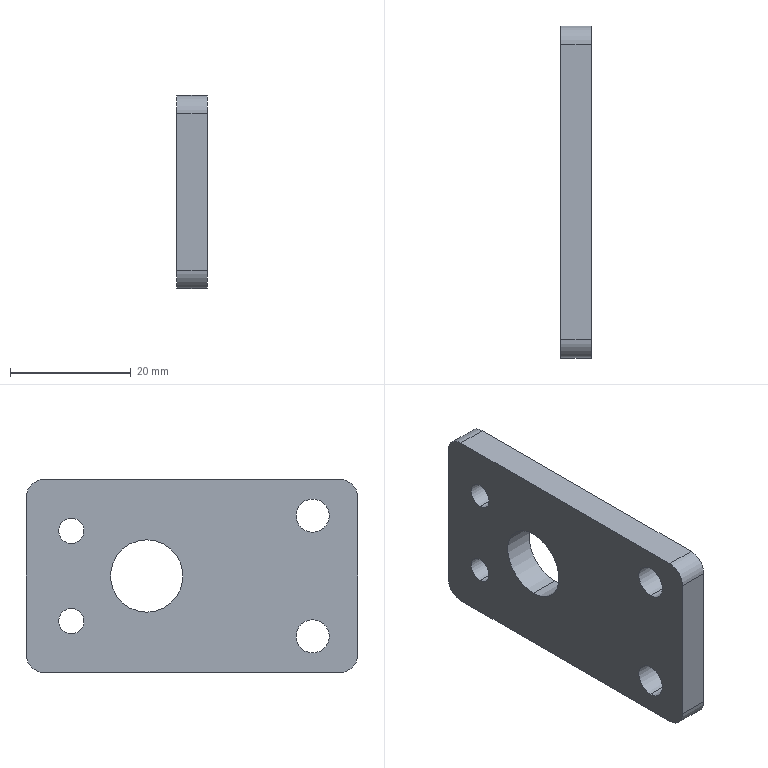Part | SolidWorks | features HoleWzd 2, Cut 1, Fillet 1, FlatPattern 1, SMBaseFlange 1, SheetMetal 1 | 1 solid | 20 faces | box 5 x 55 x 32 mm | volume 7820 mm3 | cylinder 14 | plane 6 | commonest cylinder face diameters 4.2 x4 5.5 x4 6 x4 12 x2
STEP:
#1=CARTESIAN_POINT('',(-5.,7.5,6.));
#2=VERTEX_POINT('',#1);
#3=CARTESIAN_POINT('',(-5.,7.5,-6.));
#4=VERTEX_POINT('',#3);
#5=CARTESIAN_POINT('',(-5.,7.5,0.));
#6=DIRECTION('',(1.,0.,0.));
#7=DIRECTION('',(0.,0.,-1.));
#8=AXIS2_PLACEMENT_3D('',#5,#6,#7);
#9=CIRCLE('',#8,6.);
#10=EDGE_CURVE('',#2,#4,#9,.T.);
#11=ORIENTED_EDGE('',*,*,#10,.F.);
#12=CARTESIAN_POINT('',(0.,7.5,6.));
#13=VERTEX_POINT('',#12);
#14=CARTESIAN_POINT('',(-5.,7.5,6.));
#15=DIRECTION('',(1.,0.,0.));
#16=VECTOR('',#15,1000.);
#17=LINE('',#14,#16);
#18=EDGE_CURVE('',#2,#13,#17,.T.);
#19=ORIENTED_EDGE('',*,*,#18,.T.);
#20=CARTESIAN_POINT('',(0.,7.5,-6.));
#21=VERTEX_POINT('',#20);
#22=CARTESIAN_POINT('',(0.,7.5,0.));
#23=DIRECTION('',(1.,0.,0.));
#24=DIRECTION('',(0.,0.,-1.));
#25=AXIS2_PLACEMENT_3D('',#22,#23,#24);
#26=CIRCLE('',#25,6.);
#27=EDGE_CURVE('',#13,#21,#26,.T.);
#28=ORIENTED_EDGE('',*,*,#27,.T.);
#29=CARTESIAN_POINT('',(-5.,7.5,-6.));
#30=DIRECTION('',(1.,0.,0.));
#31=VECTOR('',#30,1000.);
#32=LINE('',#29,#31);
#33=EDGE_CURVE('',#4,#21,#32,.T.);
#34=ORIENTED_EDGE('',*,*,#33,.F.);
#35=EDGE_LOOP('',(#11,#19,#28,#34));
#36=FACE_OUTER_BOUND('',#35,.T.);
#37=CARTESIAN_POINT('',(-5.,7.5,0.));
#38=DIRECTION('',(1.,0.,0.));
#39=DIRECTION('',(0.,0.,-1.));
#40=AXIS2_PLACEMENT_3D('',#37,#38,#39);
#41=CYLINDRICAL_SURFACE('',#40,6.);
#42=ADVANCED_FACE('',(#36),#41,.F.);
#43=CARTESIAN_POINT('',(0.,20.,-9.6));
#44=VERTEX_POINT('',#43);
#45=CARTESIAN_POINT('',(0.,20.,-5.4));
#46=VERTEX_POINT('',#45);
#47=CARTESIAN_POINT('',(0.,20.,-7.5));
#48=DIRECTION('',(-1.,0.,0.));
#49=DIRECTION('',(0.,0.,1.));
#50=AXIS2_PLACEMENT_3D('',#47,#48,#49);
#51=CIRCLE('',#50,2.1);
#52=EDGE_CURVE('',#44,#46,#51,.T.);
#53=ORIENTED_EDGE('',*,*,#52,.F.);
#54=CARTESIAN_POINT('',(-5.,20.,-9.6));
#55=VERTEX_POINT('',#54);
#56=CARTESIAN_POINT('',(-5.,20.,-9.6));
#57=DIRECTION('',(-1.,0.,0.));
#58=VECTOR('',#57,1000.);
#59=LINE('',#56,#58);
#60=EDGE_CURVE('',#44,#55,#59,.T.);
#61=ORIENTED_EDGE('',*,*,#60,.T.);
#62=CARTESIAN_POINT('',(-5.,20.,-5.4));
#63=VERTEX_POINT('',#62);
#64=CARTESIAN_POINT('',(-5.,20.,-7.5));
#65=DIRECTION('',(-1.,0.,0.));
#66=DIRECTION('',(0.,0.,1.));
#67=AXIS2_PLACEMENT_3D('',#64,#65,#66);
#68=CIRCLE('',#67,2.1);
#69=EDGE_CURVE('',#55,#63,#68,.T.);
#70=ORIENTED_EDGE('',*,*,#69,.T.);
#71=CARTESIAN_POINT('',(-5.,20.,-5.4));
#72=DIRECTION('',(-1.,0.,0.));
#73=VECTOR('',#72,1000.);
#74=LINE('',#71,#73);
#75=EDGE_CURVE('',#46,#63,#74,.T.);
#76=ORIENTED_EDGE('',*,*,#75,.F.);
#77=EDGE_LOOP('',(#53,#61,#70,#76));
#78=FACE_OUTER_BOUND('',#77,.T.);
#79=CARTESIAN_POINT('',(-5.,20.,-7.5));
#80=DIRECTION('',(-1.,0.,0.));
#81=DIRECTION('',(0.,0.,1.));
#82=AXIS2_PLACEMENT_3D('',#79,#80,#81);
#83=CYLINDRICAL_SURFACE('',#82,2.1);
#84=ADVANCED_FACE('',(#78),#83,.F.);
#85=CARTESIAN_POINT('',(0.,20.,5.4));
#86=VERTEX_POINT('',#85);
#87=CARTESIAN_POINT('',(0.,20.,9.6));
#88=VERTEX_POINT('',#87);
#89=CARTESIAN_POINT('',(0.,20.,7.5));
#90=DIRECTION('',(-1.,0.,0.));
#91=DIRECTION('',(0.,0.,1.));
#92=AXIS2_PLACEMENT_3D('',#89,#90,#91);
#93=CIRCLE('',#92,2.1);
#94=EDGE_CURVE('',#86,#88,#93,.T.);
#95=ORIENTED_EDGE('',*,*,#94,.F.);
#96=CARTESIAN_POINT('',(-5.,20.,5.4));
#97=VERTEX_POINT('',#96);
#98=CARTESIAN_POINT('',(-5.,20.,5.4));
#99=DIRECTION('',(-1.,0.,0.));
#100=VECTOR('',#99,1000.);
#101=LINE('',#98,#100);
#102=EDGE_CURVE('',#86,#97,#101,.T.);
#103=ORIENTED_EDGE('',*,*,#102,.T.);
#104=CARTESIAN_POINT('',(-5.,20.,9.6));
#105=VERTEX_POINT('',#104);
#106=CARTESIAN_POINT('',(-5.,20.,7.5));
#107=DIRECTION('',(-1.,0.,0.));
#108=DIRECTION('',(0.,0.,1.));
#109=AXIS2_PLACEMENT_3D('',#106,#107,#108);
#110=CIRCLE('',#109,2.1);
#111=EDGE_CURVE('',#97,#105,#110,.T.);
#112=ORIENTED_EDGE('',*,*,#111,.T.);
#113=CARTESIAN_POINT('',(-5.,20.,9.6));
#114=DIRECTION('',(-1.,0.,0.));
#115=VECTOR('',#114,1000.);
#116=LINE('',#113,#115);
#117=EDGE_CURVE('',#88,#105,#116,.T.);
#118=ORIENTED_EDGE('',*,*,#117,.F.);
#119=EDGE_LOOP('',(#95,#103,#112,#118));
#120=FACE_OUTER_BOUND('',#119,.T.);
#121=CARTESIAN_POINT('',(-5.,20.,7.5));
#122=DIRECTION('',(-1.,0.,0.));
#123=DIRECTION('',(0.,0.,1.));
#124=AXIS2_PLACEMENT_3D('',#121,#122,#123);
#125=CYLINDRICAL_SURFACE('',#124,2.1);
#126=ADVANCED_FACE('',(#120),#125,.F.);
#127=CARTESIAN_POINT('',(-5.,-20.,7.25));
#128=VERTEX_POINT('',#127);
#129=CARTESIAN_POINT('',(-5.,-20.,12.75));
#130=VERTEX_POINT('',#129);
#131=CARTESIAN_POINT('',(-5.,-20.,10.));
#132=DIRECTION('',(-1.,0.,0.));
#133=DIRECTION('',(0.,0.,1.));
#134=AXIS2_PLACEMENT_3D('',#131,#132,#133);
#135=CIRCLE('',#134,2.75);
#136=EDGE_CURVE('',#128,#130,#135,.T.);
#137=ORIENTED_EDGE('',*,*,#136,.T.);
#138=CARTESIAN_POINT('',(0.,-20.,12.75));
#139=VERTEX_POINT('',#138);
#140=CARTESIAN_POINT('',(0.,-20.,12.75));
#141=DIRECTION('',(1.,0.,0.));
#142=VECTOR('',#141,1000.);
#143=LINE('',#140,#142);
#144=EDGE_CURVE('',#130,#139,#143,.T.);
#145=ORIENTED_EDGE('',*,*,#144,.T.);
#146=CARTESIAN_POINT('',(0.,-20.,7.25));
#147=VERTEX_POINT('',#146);
#148=CARTESIAN_POINT('',(0.,-20.,10.));
#149=DIRECTION('',(1.,0.,0.));
#150=DIRECTION('',(0.,0.,-1.));
#151=AXIS2_PLACEMENT_3D('',#148,#149,#150);
#152=CIRCLE('',#151,2.75);
#153=EDGE_CURVE('',#139,#147,#152,.T.);
#154=ORIENTED_EDGE('',*,*,#153,.T.);
#155=CARTESIAN_POINT('',(0.,-20.,7.25));
#156=DIRECTION('',(1.,0.,0.));
#157=VECTOR('',#156,1000.);
#158=LINE('',#155,#157);
#159=EDGE_CURVE('',#128,#147,#158,.T.);
#160=ORIENTED_EDGE('',*,*,#159,.F.);
#161=EDGE_LOOP('',(#137,#145,#154,#160));
#162=FACE_OUTER_BOUND('',#161,.T.);
#163=CARTESIAN_POINT('',(0.,-20.,10.));
#164=DIRECTION('',(1.,0.,0.));
#165=DIRECTION('',(0.,0.,-1.));
#166=AXIS2_PLACEMENT_3D('',#163,#164,#165);
#167=CYLINDRICAL_SURFACE('',#166,2.75);
#168=ADVANCED_FACE('',(#162),#167,.F.);
#169=CARTESIAN_POINT('',(-5.,-20.,-12.75));
#170=VERTEX_POINT('',#169);
#171=CARTESIAN_POINT('',(-5.,-20.,-7.25));
#172=VERTEX_POINT('',#171);
#173=CARTESIAN_POINT('',(-5.,-20.,-10.));
#174=DIRECTION('',(-1.,0.,0.));
#175=DIRECTION('',(0.,0.,1.));
#176=AXIS2_PLACEMENT_3D('',#173,#174,#175);
#177=CIRCLE('',#176,2.75);
#178=EDGE_CURVE('',#170,#172,#177,.T.);
#179=ORIENTED_EDGE('',*,*,#178,.T.);
#180=CARTESIAN_POINT('',(0.,-20.,-7.25));
#181=VERTEX_POINT('',#180);
#182=CARTESIAN_POINT('',(0.,-20.,-7.25));
#183=DIRECTION('',(1.,0.,0.));
#184=VECTOR('',#183,1000.);
#185=LINE('',#182,#184);
#186=EDGE_CURVE('',#172,#181,#185,.T.);
#187=ORIENTED_EDGE('',*,*,#186,.T.);
#188=CARTESIAN_POINT('',(0.,-20.,-12.75));
#189=VERTEX_POINT('',#188);
#190=CARTESIAN_POINT('',(0.,-20.,-10.));
#191=DIRECTION('',(1.,0.,0.));
#192=DIRECTION('',(0.,0.,-1.));
#193=AXIS2_PLACEMENT_3D('',#190,#191,#192);
#194=CIRCLE('',#193,2.75);
#195=EDGE_CURVE('',#181,#189,#194,.T.);
#196=ORIENTED_EDGE('',*,*,#195,.T.);
#197=CARTESIAN_POINT('',(0.,-20.,-12.75));
#198=DIRECTION('',(1.,0.,0.));
#199=VECTOR('',#198,1000.);
#200=LINE('',#197,#199);
#201=EDGE_CURVE('',#170,#189,#200,.T.);
#202=ORIENTED_EDGE('',*,*,#201,.F.);
#203=EDGE_LOOP('',(#179,#187,#196,#202));
#204=FACE_OUTER_BOUND('',#203,.T.);
#205=CARTESIAN_POINT('',(0.,-20.,-10.));
#206=DIRECTION('',(1.,0.,0.));
#207=DIRECTION('',(0.,0.,-1.));
#208=AXIS2_PLACEMENT_3D('',#205,#206,#207);
#209=CYLINDRICAL_SURFACE('',#208,2.75);
#210=ADVANCED_FACE('',(#204),#209,.F.);
#211=CARTESIAN_POINT('',(0.,-24.5,-16.));
#212=VERTEX_POINT('',#211);
#213=CARTESIAN_POINT('',(0.,24.5,-16.));
#214=VERTEX_POINT('',#213);
#215=CARTESIAN_POINT('',(0.,-27.5,-16.));
#216=DIRECTION('',(0.,1.,0.));
#217=VECTOR('',#216,1000.);
#218=LINE('',#215,#217);
#219=EDGE_CURVE('',#212,#214,#218,.T.);
#220=ORIENTED_EDGE('',*,*,#219,.F.);
#221=CARTESIAN_POINT('',(-5.,-24.5,-16.));
#222=VERTEX_POINT('',#221);
#223=CARTESIAN_POINT('',(-5.,-24.5,-16.));
#224=DIRECTION('',(-1.,0.,0.));
#225=VECTOR('',#224,1000.);
#226=LINE('',#223,#225);
#227=EDGE_CURVE('',#212,#222,#226,.T.);
#228=ORIENTED_EDGE('',*,*,#227,.T.);
#229=CARTESIAN_POINT('',(-5.,24.5,-16.));
#230=VERTEX_POINT('',#229);
#231=CARTESIAN_POINT('',(-5.,-27.5,-16.));
#232=DIRECTION('',(0.,1.,0.));
#233=VECTOR('',#232,1000.);
#234=LINE('',#231,#233);
#235=EDGE_CURVE('',#222,#230,#234,.T.);
#236=ORIENTED_EDGE('',*,*,#235,.T.);
#237=CARTESIAN_POINT('',(-5.,24.5,-16.));
#238=DIRECTION('',(1.,0.,0.));
#239=VECTOR('',#238,1000.);
#240=LINE('',#237,#239);
#241=EDGE_CURVE('',#230,#214,#240,.T.);
#242=ORIENTED_EDGE('',*,*,#241,.T.);
#243=EDGE_LOOP('',(#220,#228,#236,#242));
#244=FACE_OUTER_BOUND('',#243,.T.);
#245=CARTESIAN_POINT('',(-5.,-27.5,-16.));
#246=DIRECTION('',(0.,0.,-1.));
#247=DIRECTION('',(-1.,0.,0.));
#248=AXIS2_PLACEMENT_3D('',#245,#246,#247);
#249=PLANE('',#248);
#250=ADVANCED_FACE('',(#244),#249,.T.);
#251=CARTESIAN_POINT('',(-5.,-27.5,13.));
#252=VERTEX_POINT('',#251);
#253=CARTESIAN_POINT('',(-5.,-27.5,-13.));
#254=VERTEX_POINT('',#253);
#255=CARTESIAN_POINT('',(-5.,-27.5,16.));
#256=DIRECTION('',(0.,0.,-1.));
#257=VECTOR('',#256,1000.);
#258=LINE('',#255,#257);
#259=EDGE_CURVE('',#252,#254,#258,.T.);
#260=ORIENTED_EDGE('',*,*,#259,.T.);
#261=CARTESIAN_POINT('',(0.,-27.5,-13.));
#262=VERTEX_POINT('',#261);
#263=CARTESIAN_POINT('',(-5.,-27.5,-13.));
#264=DIRECTION('',(1.,0.,0.));
#265=VECTOR('',#264,1000.);
#266=LINE('',#263,#265);
#267=EDGE_CURVE('',#254,#262,#266,.T.);
#268=ORIENTED_EDGE('',*,*,#267,.T.);
#269=CARTESIAN_POINT('',(0.,-27.5,13.));
#270=VERTEX_POINT('',#269);
#271=CARTESIAN_POINT('',(0.,-27.5,16.));
#272=DIRECTION('',(0.,0.,-1.));
#273=VECTOR('',#272,1000.);
#274=LINE('',#271,#273);
#275=EDGE_CURVE('',#270,#262,#274,.T.);
#276=ORIENTED_EDGE('',*,*,#275,.F.);
#277=CARTESIAN_POINT('',(-5.,-27.5,13.));
#278=DIRECTION('',(-1.,0.,0.));
#279=VECTOR('',#278,1000.);
#280=LINE('',#277,#279);
#281=EDGE_CURVE('',#270,#252,#280,.T.);
#282=ORIENTED_EDGE('',*,*,#281,.T.);
#283=EDGE_LOOP('',(#260,#268,#276,#282));
#284=FACE_OUTER_BOUND('',#283,.T.);
#285=CARTESIAN_POINT('',(-5.,-27.5,16.));
#286=DIRECTION('',(0.,-1.,0.));
#287=DIRECTION('',(0.,0.,-1.));
#288=AXIS2_PLACEMENT_3D('',#285,#286,#287);
#289=PLANE('',#288);
#290=ADVANCED_FACE('',(#284),#289,.T.);
#291=CARTESIAN_POINT('',(-5.,24.5,16.));
#292=VERTEX_POINT('',#291);
#293=CARTESIAN_POINT('',(-5.,-24.5,16.));
#294=VERTEX_POINT('',#293);
#295=CARTESIAN_POINT('',(-5.,-27.5,16.));
#296=DIRECTION('',(0.,-1.,0.));
#297=VECTOR('',#296,1000.);
#298=LINE('',#295,#297);
#299=EDGE_CURVE('',#292,#294,#298,.T.);
#300=ORIENTED_EDGE('',*,*,#299,.T.);
#301=CARTESIAN_POINT('',(0.,-24.5,16.));
#302=VERTEX_POINT('',#301);
#303=CARTESIAN_POINT('',(-5.,-24.5,16.));
#304=DIRECTION('',(1.,0.,0.));
#305=VECTOR('',#304,1000.);
#306=LINE('',#303,#305);
#307=EDGE_CURVE('',#294,#302,#306,.T.);
#308=ORIENTED_EDGE('',*,*,#307,.T.);
#309=CARTESIAN_POINT('',(0.,24.5,16.));
#310=VERTEX_POINT('',#309);
#311=CARTESIAN_POINT('',(0.,-27.5,16.));
#312=DIRECTION('',(0.,-1.,0.));
#313=VECTOR('',#312,1000.);
#314=LINE('',#311,#313);
#315=EDGE_CURVE('',#310,#302,#314,.T.);
#316=ORIENTED_EDGE('',*,*,#315,.F.);
#317=CARTESIAN_POINT('',(-5.,24.5,16.));
#318=DIRECTION('',(-1.,0.,0.));
#319=VECTOR('',#318,1000.);
#320=LINE('',#317,#319);
#321=EDGE_CURVE('',#310,#292,#320,.T.);
#322=ORIENTED_EDGE('',*,*,#321,.T.);
#323=EDGE_LOOP('',(#300,#308,#316,#322));
#324=FACE_OUTER_BOUND('',#323,.T.);
#325=CARTESIAN_POINT('',(-5.,-27.5,16.));
#326=DIRECTION('',(0.,0.,1.));
#327=DIRECTION('',(1.,0.,0.));
#328=AXIS2_PLACEMENT_3D('',#325,#326,#327);
#329=PLANE('',#328);
#330=ADVANCED_FACE('',(#324),#329,.T.);
#331=CARTESIAN_POINT('',(0.,27.5,-13.));
#332=VERTEX_POINT('',#331);
#333=CARTESIAN_POINT('',(0.,27.5,13.));
#334=VERTEX_POINT('',#333);
#335=CARTESIAN_POINT('',(0.,27.5,16.));
#336=DIRECTION('',(0.,0.,1.));
#337=VECTOR('',#336,1000.);
#338=LINE('',#335,#337);
#339=EDGE_CURVE('',#332,#334,#338,.T.);
#340=ORIENTED_EDGE('',*,*,#339,.F.);
#341=CARTESIAN_POINT('',(-5.,27.5,-13.));
#342=VERTEX_POINT('',#341);
#343=CARTESIAN_POINT('',(-5.,27.5,-13.));
#344=DIRECTION('',(-1.,0.,0.));
#345=VECTOR('',#344,1000.);
#346=LINE('',#343,#345);
#347=EDGE_CURVE('',#332,#342,#346,.T.);
#348=ORIENTED_EDGE('',*,*,#347,.T.);
#349=CARTESIAN_POINT('',(-5.,27.5,13.));
#350=VERTEX_POINT('',#349);
#351=CARTESIAN_POINT('',(-5.,27.5,16.));
#352=DIRECTION('',(0.,0.,1.));
#353=VECTOR('',#352,1000.);
#354=LINE('',#351,#353);
#355=EDGE_CURVE('',#342,#350,#354,.T.);
#356=ORIENTED_EDGE('',*,*,#355,.T.);
#357=CARTESIAN_POINT('',(-5.,27.5,13.));
#358=DIRECTION('',(1.,0.,0.));
#359=VECTOR('',#358,1000.);
#360=LINE('',#357,#359);
#361=EDGE_CURVE('',#350,#334,#360,.T.);
#362=ORIENTED_EDGE('',*,*,#361,.T.);
#363=EDGE_LOOP('',(#340,#348,#356,#362));
#364=FACE_OUTER_BOUND('',#363,.T.);
#365=CARTESIAN_POINT('',(-5.,27.5,16.));
#366=DIRECTION('',(0.,1.,0.));
#367=DIRECTION('',(0.,0.,1.));
#368=AXIS2_PLACEMENT_3D('',#365,#366,#367);
#369=PLANE('',#368);
#370=ADVANCED_FACE('',(#364),#369,.T.);
#371=CARTESIAN_POINT('',(-5.,7.5,0.));
#372=DIRECTION('',(1.,0.,0.));
#373=DIRECTION('',(0.,0.,-1.));
#374=AXIS2_PLACEMENT_3D('',#371,#372,#373);
#375=CIRCLE('',#374,6.);
#376=EDGE_CURVE('',#4,#2,#375,.T.);
#377=ORIENTED_EDGE('',*,*,#376,.T.);
#378=ORIENTED_EDGE('',*,*,#10,.T.);
#379=EDGE_LOOP('',(#377,#378));
#380=FACE_BOUND('',#379,.T.);
#381=CARTESIAN_POINT('',(-5.,20.,-7.5));
#382=DIRECTION('',(-1.,0.,0.));
#383=DIRECTION('',(0.,0.,1.));
#384=AXIS2_PLACEMENT_3D('',#381,#382,#383);
#385=CIRCLE('',#384,2.1);
#386=EDGE_CURVE('',#63,#55,#385,.T.);
#387=ORIENTED_EDGE('',*,*,#386,.F.);
#388=ORIENTED_EDGE('',*,*,#69,.F.);
#389=EDGE_LOOP('',(#387,#388));
#390=FACE_BOUND('',#389,.T.);
#391=CARTESIAN_POINT('',(-5.,20.,7.5));
#392=DIRECTION('',(-1.,0.,0.));
#393=DIRECTION('',(0.,0.,1.));
#394=AXIS2_PLACEMENT_3D('',#391,#392,#393);
#395=CIRCLE('',#394,2.1);
#396=EDGE_CURVE('',#105,#97,#395,.T.);
#397=ORIENTED_EDGE('',*,*,#396,.F.);
#398=ORIENTED_EDGE('',*,*,#111,.F.);
#399=EDGE_LOOP('',(#397,#398));
#400=FACE_BOUND('',#399,.T.);
#401=ORIENTED_EDGE('',*,*,#136,.F.);
#402=CARTESIAN_POINT('',(-5.,-20.,10.));
#403=DIRECTION('',(-1.,0.,0.));
#404=DIRECTION('',(0.,0.,1.));
#405=AXIS2_PLACEMENT_3D('',#402,#403,#404);
#406=CIRCLE('',#405,2.75);
#407=EDGE_CURVE('',#130,#128,#406,.T.);
#408=ORIENTED_EDGE('',*,*,#407,.F.);
#409=EDGE_LOOP('',(#401,#408));
#410=FACE_BOUND('',#409,.T.);
#411=ORIENTED_EDGE('',*,*,#178,.F.);
#412=CARTESIAN_POINT('',(-5.,-20.,-10.));
#413=DIRECTION('',(-1.,0.,0.));
#414=DIRECTION('',(0.,0.,1.));
#415=AXIS2_PLACEMENT_3D('',#412,#413,#414);
#416=CIRCLE('',#415,2.75);
#417=EDGE_CURVE('',#172,#170,#416,.T.);
#418=ORIENTED_EDGE('',*,*,#417,.F.);
#419=EDGE_LOOP('',(#411,#418));
#420=FACE_BOUND('',#419,.T.);
#421=ORIENTED_EDGE('',*,*,#235,.F.);
#422=CARTESIAN_POINT('',(-5.,-24.5,-13.));
#423=DIRECTION('',(-1.,0.,0.));
#424=DIRECTION('',(0.,0.,1.));
#425=AXIS2_PLACEMENT_3D('',#422,#423,#424);
#426=CIRCLE('',#425,3.);
#427=EDGE_CURVE('',#222,#254,#426,.T.);
#428=ORIENTED_EDGE('',*,*,#427,.T.);
#429=ORIENTED_EDGE('',*,*,#259,.F.);
#430=CARTESIAN_POINT('',(-5.,-24.5,13.));
#431=DIRECTION('',(-1.,0.,0.));
#432=DIRECTION('',(0.,0.,1.));
#433=AXIS2_PLACEMENT_3D('',#430,#431,#432);
#434=CIRCLE('',#433,3.);
#435=EDGE_CURVE('',#252,#294,#434,.T.);
#436=ORIENTED_EDGE('',*,*,#435,.T.);
#437=ORIENTED_EDGE('',*,*,#299,.F.);
#438=CARTESIAN_POINT('',(-5.,24.5,13.));
#439=DIRECTION('',(-1.,0.,0.));
#440=DIRECTION('',(0.,0.,1.));
#441=AXIS2_PLACEMENT_3D('',#438,#439,#440);
#442=CIRCLE('',#441,3.);
#443=EDGE_CURVE('',#292,#350,#442,.T.);
#444=ORIENTED_EDGE('',*,*,#443,.T.);
#445=ORIENTED_EDGE('',*,*,#355,.F.);
#446=CARTESIAN_POINT('',(-5.,24.5,-13.));
#447=DIRECTION('',(-1.,0.,0.));
#448=DIRECTION('',(0.,0.,1.));
#449=AXIS2_PLACEMENT_3D('',#446,#447,#448);
#450=CIRCLE('',#449,3.);
#451=EDGE_CURVE('',#342,#230,#450,.T.);
#452=ORIENTED_EDGE('',*,*,#451,.T.);
#453=EDGE_LOOP('',(#421,#428,#429,#436,#437,#444,#445,#452));
#454=FACE_OUTER_BOUND('',#453,.T.);
#455=CARTESIAN_POINT('',(-5.,0.,0.));
#456=DIRECTION('',(-1.,0.,0.));
#457=DIRECTION('',(0.,0.,1.));
#458=AXIS2_PLACEMENT_3D('',#455,#456,#457);
#459=PLANE('',#458);
#460=ADVANCED_FACE('',(#380,#390,#400,#410,#420,#454),#459,.T.);
#461=CARTESIAN_POINT('',(0.,7.5,0.));
#462=DIRECTION('',(1.,0.,0.));
#463=DIRECTION('',(0.,0.,-1.));
#464=AXIS2_PLACEMENT_3D('',#461,#462,#463);
#465=CIRCLE('',#464,6.);
#466=EDGE_CURVE('',#21,#13,#465,.T.);
#467=ORIENTED_EDGE('',*,*,#466,.F.);
#468=ORIENTED_EDGE('',*,*,#27,.F.);
#469=EDGE_LOOP('',(#467,#468));
#470=FACE_BOUND('',#469,.T.);
#471=CARTESIAN_POINT('',(0.,20.,-7.5));
#472=DIRECTION('',(-1.,0.,0.));
#473=DIRECTION('',(0.,0.,1.));
#474=AXIS2_PLACEMENT_3D('',#471,#472,#473);
#475=CIRCLE('',#474,2.1);
#476=EDGE_CURVE('',#46,#44,#475,.T.);
#477=ORIENTED_EDGE('',*,*,#476,.T.);
#478=ORIENTED_EDGE('',*,*,#52,.T.);
#479=EDGE_LOOP('',(#477,#478));
#480=FACE_BOUND('',#479,.T.);
#481=CARTESIAN_POINT('',(0.,20.,7.5));
#482=DIRECTION('',(-1.,0.,0.));
#483=DIRECTION('',(0.,0.,1.));
#484=AXIS2_PLACEMENT_3D('',#481,#482,#483);
#485=CIRCLE('',#484,2.1);
#486=EDGE_CURVE('',#88,#86,#485,.T.);
#487=ORIENTED_EDGE('',*,*,#486,.T.);
#488=ORIENTED_EDGE('',*,*,#94,.T.);
#489=EDGE_LOOP('',(#487,#488));
#490=FACE_BOUND('',#489,.T.);
#491=CARTESIAN_POINT('',(0.,-20.,10.));
#492=DIRECTION('',(1.,0.,0.));
#493=DIRECTION('',(0.,0.,-1.));
#494=AXIS2_PLACEMENT_3D('',#491,#492,#493);
#495=CIRCLE('',#494,2.75);
#496=EDGE_CURVE('',#147,#139,#495,.T.);
#497=ORIENTED_EDGE('',*,*,#496,.F.);
#498=ORIENTED_EDGE('',*,*,#153,.F.);
#499=EDGE_LOOP('',(#497,#498));
#500=FACE_BOUND('',#499,.T.);
#501=CARTESIAN_POINT('',(0.,-20.,-10.));
#502=DIRECTION('',(1.,0.,0.));
#503=DIRECTION('',(0.,0.,-1.));
#504=AXIS2_PLACEMENT_3D('',#501,#502,#503);
#505=CIRCLE('',#504,2.75);
#506=EDGE_CURVE('',#189,#181,#505,.T.);
#507=ORIENTED_EDGE('',*,*,#506,.F.);
#508=ORIENTED_EDGE('',*,*,#195,.F.);
#509=EDGE_LOOP('',(#507,#508));
#510=FACE_BOUND('',#509,.T.);
#511=ORIENTED_EDGE('',*,*,#275,.T.);
#512=CARTESIAN_POINT('',(0.,-24.5,-13.));
#513=DIRECTION('',(1.,0.,0.));
#514=DIRECTION('',(0.,0.,1.));
#515=AXIS2_PLACEMENT_3D('',#512,#513,#514);
#516=CIRCLE('',#515,3.);
#517=EDGE_CURVE('',#262,#212,#516,.T.);
#518=ORIENTED_EDGE('',*,*,#517,.T.);
#519=ORIENTED_EDGE('',*,*,#219,.T.);
#520=CARTESIAN_POINT('',(0.,24.5,-13.));
#521=DIRECTION('',(1.,0.,0.));
#522=DIRECTION('',(0.,0.,1.));
#523=AXIS2_PLACEMENT_3D('',#520,#521,#522);
#524=CIRCLE('',#523,3.);
#525=EDGE_CURVE('',#214,#332,#524,.T.);
#526=ORIENTED_EDGE('',*,*,#525,.T.);
#527=ORIENTED_EDGE('',*,*,#339,.T.);
#528=CARTESIAN_POINT('',(0.,24.5,13.));
#529=DIRECTION('',(1.,0.,0.));
#530=DIRECTION('',(0.,0.,1.));
#531=AXIS2_PLACEMENT_3D('',#528,#529,#530);
#532=CIRCLE('',#531,3.);
#533=EDGE_CURVE('',#334,#310,#532,.T.);
#534=ORIENTED_EDGE('',*,*,#533,.T.);
#535=ORIENTED_EDGE('',*,*,#315,.T.);
#536=CARTESIAN_POINT('',(0.,-24.5,13.));
#537=DIRECTION('',(1.,0.,0.));
#538=DIRECTION('',(0.,0.,1.));
#539=AXIS2_PLACEMENT_3D('',#536,#537,#538);
#540=CIRCLE('',#539,3.);
#541=EDGE_CURVE('',#302,#270,#540,.T.);
#542=ORIENTED_EDGE('',*,*,#541,.T.);
#543=EDGE_LOOP('',(#511,#518,#519,#526,#527,#534,#535,#542));
#544=FACE_OUTER_BOUND('',#543,.T.);
#545=CARTESIAN_POINT('',(0.,0.,0.));
#546=DIRECTION('',(-1.,0.,0.));
#547=DIRECTION('',(0.,0.,1.));
#548=AXIS2_PLACEMENT_3D('',#545,#546,#547);
#549=PLANE('',#548);
#550=ADVANCED_FACE('',(#470,#480,#490,#500,#510,#544),#549,.F.);
#551=ORIENTED_EDGE('',*,*,#186,.F.);
#552=ORIENTED_EDGE('',*,*,#417,.T.);
#553=ORIENTED_EDGE('',*,*,#201,.T.);
#554=ORIENTED_EDGE('',*,*,#506,.T.);
#555=EDGE_LOOP('',(#551,#552,#553,#554));
#556=FACE_OUTER_BOUND('',#555,.T.);
#557=CARTESIAN_POINT('',(0.,-20.,-10.));
#558=DIRECTION('',(1.,0.,0.));
#559=DIRECTION('',(0.,0.,-1.));
#560=AXIS2_PLACEMENT_3D('',#557,#558,#559);
#561=CYLINDRICAL_SURFACE('',#560,2.75);
#562=ADVANCED_FACE('',(#556),#561,.F.);
#563=ORIENTED_EDGE('',*,*,#144,.F.);
#564=ORIENTED_EDGE('',*,*,#407,.T.);
#565=ORIENTED_EDGE('',*,*,#159,.T.);
#566=ORIENTED_EDGE('',*,*,#496,.T.);
#567=EDGE_LOOP('',(#563,#564,#565,#566));
#568=FACE_OUTER_BOUND('',#567,.T.);
#569=CARTESIAN_POINT('',(0.,-20.,10.));
#570=DIRECTION('',(1.,0.,0.));
#571=DIRECTION('',(0.,0.,-1.));
#572=AXIS2_PLACEMENT_3D('',#569,#570,#571);
#573=CYLINDRICAL_SURFACE('',#572,2.75);
#574=ADVANCED_FACE('',(#568),#573,.F.);
#575=ORIENTED_EDGE('',*,*,#102,.F.);
#576=ORIENTED_EDGE('',*,*,#486,.F.);
#577=ORIENTED_EDGE('',*,*,#117,.T.);
#578=ORIENTED_EDGE('',*,*,#396,.T.);
#579=EDGE_LOOP('',(#575,#576,#577,#578));
#580=FACE_OUTER_BOUND('',#579,.T.);
#581=CARTESIAN_POINT('',(-5.,20.,7.5));
#582=DIRECTION('',(-1.,0.,0.));
#583=DIRECTION('',(0.,0.,1.));
#584=AXIS2_PLACEMENT_3D('',#581,#582,#583);
#585=CYLINDRICAL_SURFACE('',#584,2.1);
#586=ADVANCED_FACE('',(#580),#585,.F.);
#587=ORIENTED_EDGE('',*,*,#60,.F.);
#588=ORIENTED_EDGE('',*,*,#476,.F.);
#589=ORIENTED_EDGE('',*,*,#75,.T.);
#590=ORIENTED_EDGE('',*,*,#386,.T.);
#591=EDGE_LOOP('',(#587,#588,#589,#590));
#592=FACE_OUTER_BOUND('',#591,.T.);
#593=CARTESIAN_POINT('',(-5.,20.,-7.5));
#594=DIRECTION('',(-1.,0.,0.));
#595=DIRECTION('',(0.,0.,1.));
#596=AXIS2_PLACEMENT_3D('',#593,#594,#595);
#597=CYLINDRICAL_SURFACE('',#596,2.1);
#598=ADVANCED_FACE('',(#592),#597,.F.);
#599=ORIENTED_EDGE('',*,*,#427,.F.);
#600=ORIENTED_EDGE('',*,*,#227,.F.);
#601=ORIENTED_EDGE('',*,*,#517,.F.);
#602=ORIENTED_EDGE('',*,*,#267,.F.);
#603=EDGE_LOOP('',(#599,#600,#601,#602));
#604=FACE_OUTER_BOUND('',#603,.T.);
#605=CARTESIAN_POINT('',(-5.,-24.5,-13.));
#606=DIRECTION('',(1.,0.,0.));
#607=DIRECTION('',(0.,0.,-1.));
#608=AXIS2_PLACEMENT_3D('',#605,#606,#607);
#609=CYLINDRICAL_SURFACE('',#608,3.);
#610=ADVANCED_FACE('',(#604),#609,.T.);
#611=ORIENTED_EDGE('',*,*,#435,.F.);
#612=ORIENTED_EDGE('',*,*,#281,.F.);
#613=ORIENTED_EDGE('',*,*,#541,.F.);
#614=ORIENTED_EDGE('',*,*,#307,.F.);
#615=EDGE_LOOP('',(#611,#612,#613,#614));
#616=FACE_OUTER_BOUND('',#615,.T.);
#617=CARTESIAN_POINT('',(-5.,-24.5,13.));
#618=DIRECTION('',(1.,0.,0.));
#619=DIRECTION('',(0.,0.,-1.));
#620=AXIS2_PLACEMENT_3D('',#617,#618,#619);
#621=CYLINDRICAL_SURFACE('',#620,3.);
#622=ADVANCED_FACE('',(#616),#621,.T.);
#623=ORIENTED_EDGE('',*,*,#451,.F.);
#624=ORIENTED_EDGE('',*,*,#347,.F.);
#625=ORIENTED_EDGE('',*,*,#525,.F.);
#626=ORIENTED_EDGE('',*,*,#241,.F.);
#627=EDGE_LOOP('',(#623,#624,#625,#626));
#628=FACE_OUTER_BOUND('',#627,.T.);
#629=CARTESIAN_POINT('',(-5.,24.5,-13.));
#630=DIRECTION('',(1.,0.,0.));
#631=DIRECTION('',(0.,0.,-1.));
#632=AXIS2_PLACEMENT_3D('',#629,#630,#631);
#633=CYLINDRICAL_SURFACE('',#632,3.);
#634=ADVANCED_FACE('',(#628),#633,.T.);
#635=ORIENTED_EDGE('',*,*,#443,.F.);
#636=ORIENTED_EDGE('',*,*,#321,.F.);
#637=ORIENTED_EDGE('',*,*,#533,.F.);
#638=ORIENTED_EDGE('',*,*,#361,.F.);
#639=EDGE_LOOP('',(#635,#636,#637,#638));
#640=FACE_OUTER_BOUND('',#639,.T.);
#641=CARTESIAN_POINT('',(-5.,24.5,13.));
#642=DIRECTION('',(1.,0.,0.));
#643=DIRECTION('',(0.,0.,-1.));
#644=AXIS2_PLACEMENT_3D('',#641,#642,#643);
#645=CYLINDRICAL_SURFACE('',#644,3.);
#646=ADVANCED_FACE('',(#640),#645,.T.);
#647=ORIENTED_EDGE('',*,*,#18,.F.);
#648=ORIENTED_EDGE('',*,*,#376,.F.);
#649=ORIENTED_EDGE('',*,*,#33,.T.);
#650=ORIENTED_EDGE('',*,*,#466,.T.);
#651=EDGE_LOOP('',(#647,#648,#649,#650));
#652=FACE_OUTER_BOUND('',#651,.T.);
#653=CARTESIAN_POINT('',(-5.,7.5,0.));
#654=DIRECTION('',(1.,0.,0.));
#655=DIRECTION('',(0.,0.,-1.));
#656=AXIS2_PLACEMENT_3D('',#653,#654,#655);
#657=CYLINDRICAL_SURFACE('',#656,6.);
#658=ADVANCED_FACE('',(#652),#657,.F.);
#659=CLOSED_SHELL('',(#42,#84,#126,#168,#210,#250,#290,#330,#370,#460,#550,#562,#574,#586,#598,#610,#622,#634,#646,#658));
#660=MANIFOLD_SOLID_BREP('',#659);
#661=CARTESIAN_POINT('',(0.,0.,0.));
#662=DIRECTION('',(0.,0.,1.));
#663=DIRECTION('',(1.,0.,0.));
#664=AXIS2_PLACEMENT_3D('',#661,#662,#663);
#665=(LENGTH_UNIT()NAMED_UNIT(*)SI_UNIT(.MILLI.,.METRE.));
#666=UNCERTAINTY_MEASURE_WITH_UNIT(LENGTH_MEASURE(0.00001),#665,'','');
#667=(NAMED_UNIT(*)PLANE_ANGLE_UNIT()SI_UNIT($,.RADIAN.));
#668=(NAMED_UNIT(*)SI_UNIT($,.STERADIAN.)SOLID_ANGLE_UNIT());
#669=(GEOMETRIC_REPRESENTATION_CONTEXT(3)GLOBAL_UNCERTAINTY_ASSIGNED_CONTEXT((#666))GLOBAL_UNIT_ASSIGNED_CONTEXT((#665,#667,#668))REPRESENTATION_CONTEXT('',''));
#670=ADVANCED_BREP_SHAPE_REPRESENTATION('',(#660,#664),#669);